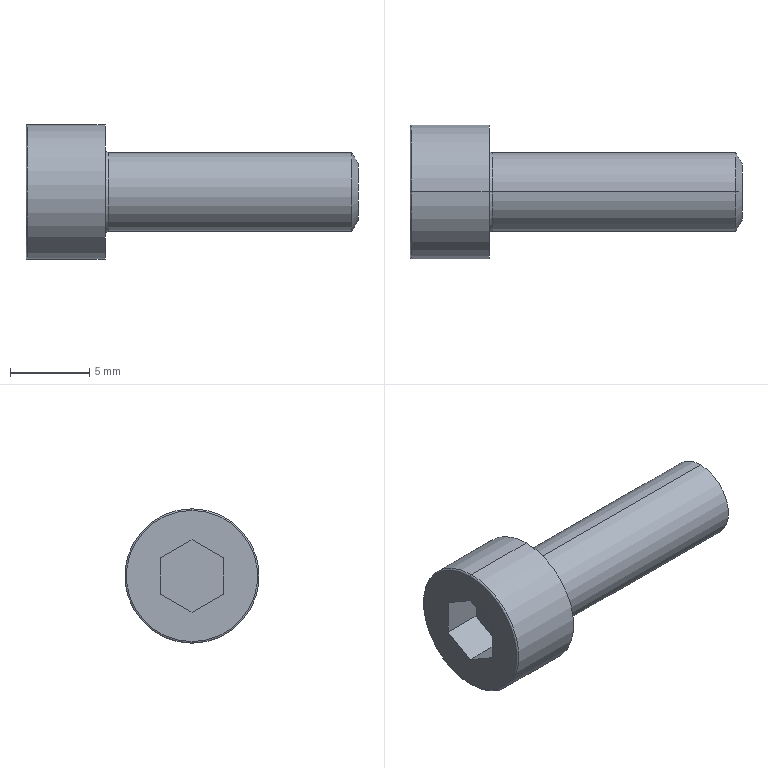Part | SolidWorks | features BlendCut 1, Cut 1, Fillet 1, LPattern 1, RevCut 1, Revolution 1 | 1 solid | 20 faces | box 21 x 8.5 x 8.5 mm | volume 561.928 mm3 | plane 10 | torus 4 | cylinder 4 | cone 2 | commonest cylinder face diameters 5 x2 8.5 x2
STEP:
#1=CARTESIAN_POINT('',(0.,0.,4.15));
#2=VERTEX_POINT('',#1);
#3=CARTESIAN_POINT('',(0.,0.,-4.15));
#4=VERTEX_POINT('',#3);
#5=CARTESIAN_POINT('',(0.,0.,0.));
#6=DIRECTION('',(-1.,0.,0.));
#7=DIRECTION('',(0.,0.,-1.));
#8=AXIS2_PLACEMENT_3D('',#5,#6,#7);
#9=CIRCLE('',#8,4.15);
#10=EDGE_CURVE('',#2,#4,#9,.T.);
#11=ORIENTED_EDGE('',*,*,#10,.F.);
#12=CARTESIAN_POINT('',(0.1,0.,4.25));
#13=VERTEX_POINT('',#12);
#14=CARTESIAN_POINT('',(0.1,0.,4.15));
#15=DIRECTION('',(0.,1.,0.));
#16=DIRECTION('',(0.,0.,1.));
#17=AXIS2_PLACEMENT_3D('',#14,#15,#16);
#18=CIRCLE('',#17,0.1);
#19=EDGE_CURVE('',#2,#13,#18,.T.);
#20=ORIENTED_EDGE('',*,*,#19,.T.);
#21=CARTESIAN_POINT('',(0.1,0.,-4.25));
#22=VERTEX_POINT('',#21);
#23=CARTESIAN_POINT('',(0.1,0.,0.));
#24=DIRECTION('',(1.,0.,0.));
#25=DIRECTION('',(0.,0.,-1.));
#26=AXIS2_PLACEMENT_3D('',#23,#24,#25);
#27=CIRCLE('',#26,4.25);
#28=EDGE_CURVE('',#22,#13,#27,.T.);
#29=ORIENTED_EDGE('',*,*,#28,.F.);
#30=CARTESIAN_POINT('',(0.1,0.,-4.15));
#31=DIRECTION('',(0.,-1.,0.));
#32=DIRECTION('',(0.,0.,-1.));
#33=AXIS2_PLACEMENT_3D('',#30,#31,#32);
#34=CIRCLE('',#33,0.1);
#35=EDGE_CURVE('',#4,#22,#34,.T.);
#36=ORIENTED_EDGE('',*,*,#35,.F.);
#37=EDGE_LOOP('',(#11,#20,#29,#36));
#38=FACE_OUTER_BOUND('',#37,.T.);
#39=CARTESIAN_POINT('',(0.1,0.,0.));
#40=DIRECTION('',(1.,0.,0.));
#41=DIRECTION('',(0.,0.,-1.));
#42=AXIS2_PLACEMENT_3D('',#39,#40,#41);
#43=TOROIDAL_SURFACE('',#42,4.15,0.1);
#44=ADVANCED_FACE('',(#38),#43,.T.);
#45=CARTESIAN_POINT('',(21.,0.,1.807));
#46=VERTEX_POINT('',#45);
#47=CARTESIAN_POINT('',(21.,0.,-1.807));
#48=VERTEX_POINT('',#47);
#49=CARTESIAN_POINT('',(21.,0.,0.));
#50=DIRECTION('',(-1.,0.,0.));
#51=DIRECTION('',(0.,0.,1.));
#52=AXIS2_PLACEMENT_3D('',#49,#50,#51);
#53=CIRCLE('',#52,1.807);
#54=EDGE_CURVE('',#46,#48,#53,.T.);
#55=ORIENTED_EDGE('',*,*,#54,.T.);
#56=CARTESIAN_POINT('',(20.6,0.,-2.5));
#57=VERTEX_POINT('',#56);
#58=CARTESIAN_POINT('',(20.6,0.,-2.5));
#59=DIRECTION('',(-0.5,0.,-0.866));
#60=VECTOR('',#59,1000.);
#61=LINE('',#58,#60);
#62=EDGE_CURVE('',#48,#57,#61,.T.);
#63=ORIENTED_EDGE('',*,*,#62,.T.);
#64=CARTESIAN_POINT('',(20.6,0.,2.5));
#65=VERTEX_POINT('',#64);
#66=CARTESIAN_POINT('',(20.6,0.,0.));
#67=DIRECTION('',(-1.,0.,0.));
#68=DIRECTION('',(0.,0.,1.));
#69=AXIS2_PLACEMENT_3D('',#66,#67,#68);
#70=CIRCLE('',#69,2.5);
#71=EDGE_CURVE('',#65,#57,#70,.T.);
#72=ORIENTED_EDGE('',*,*,#71,.F.);
#73=CARTESIAN_POINT('',(20.6,0.,2.5));
#74=DIRECTION('',(-0.5,0.,0.866));
#75=VECTOR('',#74,1000.);
#76=LINE('',#73,#75);
#77=EDGE_CURVE('',#46,#65,#76,.T.);
#78=ORIENTED_EDGE('',*,*,#77,.F.);
#79=EDGE_LOOP('',(#55,#63,#72,#78));
#80=FACE_OUTER_BOUND('',#79,.T.);
#81=CARTESIAN_POINT('',(20.6,0.,0.));
#82=DIRECTION('',(-1.,0.,0.));
#83=DIRECTION('',(0.,0.,1.));
#84=AXIS2_PLACEMENT_3D('',#81,#82,#83);
#85=CONICAL_SURFACE('',#84,2.5,1.047);
#86=ADVANCED_FACE('',(#80),#85,.T.);
#87=CARTESIAN_POINT('',(5.,0.,-2.7));
#88=VERTEX_POINT('',#87);
#89=CARTESIAN_POINT('',(5.,0.,2.7));
#90=VERTEX_POINT('',#89);
#91=CARTESIAN_POINT('',(5.,0.,0.));
#92=DIRECTION('',(-1.,0.,0.));
#93=DIRECTION('',(0.,0.,1.));
#94=AXIS2_PLACEMENT_3D('',#91,#92,#93);
#95=CIRCLE('',#94,2.7);
#96=EDGE_CURVE('',#88,#90,#95,.T.);
#97=ORIENTED_EDGE('',*,*,#96,.F.);
#98=CARTESIAN_POINT('',(5.2,0.,-2.5));
#99=VERTEX_POINT('',#98);
#100=CARTESIAN_POINT('',(5.2,0.,-2.7));
#101=DIRECTION('',(0.,1.,0.));
#102=DIRECTION('',(0.,0.,1.));
#103=AXIS2_PLACEMENT_3D('',#100,#101,#102);
#104=CIRCLE('',#103,0.2);
#105=EDGE_CURVE('',#88,#99,#104,.T.);
#106=ORIENTED_EDGE('',*,*,#105,.T.);
#107=CARTESIAN_POINT('',(5.2,0.,2.5));
#108=VERTEX_POINT('',#107);
#109=CARTESIAN_POINT('',(5.2,0.,0.));
#110=DIRECTION('',(-1.,0.,0.));
#111=DIRECTION('',(0.,0.,1.));
#112=AXIS2_PLACEMENT_3D('',#109,#110,#111);
#113=CIRCLE('',#112,2.5);
#114=EDGE_CURVE('',#99,#108,#113,.T.);
#115=ORIENTED_EDGE('',*,*,#114,.T.);
#116=CARTESIAN_POINT('',(5.2,0.,2.7));
#117=DIRECTION('',(0.,-1.,0.));
#118=DIRECTION('',(0.,0.,-1.));
#119=AXIS2_PLACEMENT_3D('',#116,#117,#118);
#120=CIRCLE('',#119,0.2);
#121=EDGE_CURVE('',#90,#108,#120,.T.);
#122=ORIENTED_EDGE('',*,*,#121,.F.);
#123=EDGE_LOOP('',(#97,#106,#115,#122));
#124=FACE_OUTER_BOUND('',#123,.T.);
#125=CARTESIAN_POINT('',(5.2,0.,0.));
#126=DIRECTION('',(-1.,0.,0.));
#127=DIRECTION('',(0.,0.,1.));
#128=AXIS2_PLACEMENT_3D('',#125,#126,#127);
#129=TOROIDAL_SURFACE('',#128,2.7,0.2);
#130=ADVANCED_FACE('',(#124),#129,.F.);
#131=CARTESIAN_POINT('',(5.,0.,4.25));
#132=VERTEX_POINT('',#131);
#133=CARTESIAN_POINT('',(5.,0.,-4.25));
#134=VERTEX_POINT('',#133);
#135=CARTESIAN_POINT('',(5.,0.,0.));
#136=DIRECTION('',(-1.,0.,0.));
#137=DIRECTION('',(0.,0.,1.));
#138=AXIS2_PLACEMENT_3D('',#135,#136,#137);
#139=CIRCLE('',#138,4.25);
#140=EDGE_CURVE('',#132,#134,#139,.T.);
#141=ORIENTED_EDGE('',*,*,#140,.T.);
#142=CARTESIAN_POINT('',(0.,0.,-4.25));
#143=DIRECTION('',(-1.,0.,0.));
#144=VECTOR('',#143,1000.);
#145=LINE('',#142,#144);
#146=EDGE_CURVE('',#134,#22,#145,.T.);
#147=ORIENTED_EDGE('',*,*,#146,.T.);
#148=ORIENTED_EDGE('',*,*,#28,.T.);
#149=CARTESIAN_POINT('',(0.,0.,4.25));
#150=DIRECTION('',(-1.,0.,0.));
#151=VECTOR('',#150,1000.);
#152=LINE('',#149,#151);
#153=EDGE_CURVE('',#132,#13,#152,.T.);
#154=ORIENTED_EDGE('',*,*,#153,.F.);
#155=EDGE_LOOP('',(#141,#147,#148,#154));
#156=FACE_OUTER_BOUND('',#155,.T.);
#157=CARTESIAN_POINT('',(0.,0.,0.));
#158=DIRECTION('',(-1.,0.,0.));
#159=DIRECTION('',(0.,0.,1.));
#160=AXIS2_PLACEMENT_3D('',#157,#158,#159);
#161=CYLINDRICAL_SURFACE('',#160,4.25);
#162=ADVANCED_FACE('',(#156),#161,.T.);
#163=ORIENTED_EDGE('',*,*,#71,.T.);
#164=CARTESIAN_POINT('',(0.,0.,-2.5));
#165=DIRECTION('',(-1.,0.,0.));
#166=VECTOR('',#165,1000.);
#167=LINE('',#164,#166);
#168=EDGE_CURVE('',#57,#99,#167,.T.);
#169=ORIENTED_EDGE('',*,*,#168,.T.);
#170=CARTESIAN_POINT('',(5.2,0.,0.));
#171=DIRECTION('',(-1.,0.,0.));
#172=DIRECTION('',(0.,0.,1.));
#173=AXIS2_PLACEMENT_3D('',#170,#171,#172);
#174=CIRCLE('',#173,2.5);
#175=EDGE_CURVE('',#108,#99,#174,.T.);
#176=ORIENTED_EDGE('',*,*,#175,.F.);
#177=CARTESIAN_POINT('',(0.,0.,2.5));
#178=DIRECTION('',(-1.,0.,0.));
#179=VECTOR('',#178,1000.);
#180=LINE('',#177,#179);
#181=EDGE_CURVE('',#65,#108,#180,.T.);
#182=ORIENTED_EDGE('',*,*,#181,.F.);
#183=EDGE_LOOP('',(#163,#169,#176,#182));
#184=FACE_OUTER_BOUND('',#183,.T.);
#185=CARTESIAN_POINT('',(0.,0.,0.));
#186=DIRECTION('',(-1.,0.,0.));
#187=DIRECTION('',(0.,0.,1.));
#188=AXIS2_PLACEMENT_3D('',#185,#186,#187);
#189=CYLINDRICAL_SURFACE('',#188,2.5);
#190=ADVANCED_FACE('',(#184),#189,.T.);
#191=ORIENTED_EDGE('',*,*,#168,.F.);
#192=CARTESIAN_POINT('',(20.6,0.,0.));
#193=DIRECTION('',(-1.,0.,0.));
#194=DIRECTION('',(0.,0.,1.));
#195=AXIS2_PLACEMENT_3D('',#192,#193,#194);
#196=CIRCLE('',#195,2.5);
#197=EDGE_CURVE('',#57,#65,#196,.T.);
#198=ORIENTED_EDGE('',*,*,#197,.T.);
#199=ORIENTED_EDGE('',*,*,#181,.T.);
#200=ORIENTED_EDGE('',*,*,#114,.F.);
#201=EDGE_LOOP('',(#191,#198,#199,#200));
#202=FACE_OUTER_BOUND('',#201,.T.);
#203=CARTESIAN_POINT('',(0.,0.,0.));
#204=DIRECTION('',(-1.,0.,0.));
#205=DIRECTION('',(0.,0.,1.));
#206=AXIS2_PLACEMENT_3D('',#203,#204,#205);
#207=CYLINDRICAL_SURFACE('',#206,2.5);
#208=ADVANCED_FACE('',(#202),#207,.T.);
#209=CARTESIAN_POINT('',(0.,0.,0.));
#210=DIRECTION('',(-1.,0.,0.));
#211=DIRECTION('',(0.,0.,-1.));
#212=AXIS2_PLACEMENT_3D('',#209,#210,#211);
#213=CIRCLE('',#212,4.15);
#214=EDGE_CURVE('',#4,#2,#213,.T.);
#215=ORIENTED_EDGE('',*,*,#214,.T.);
#216=ORIENTED_EDGE('',*,*,#10,.T.);
#217=EDGE_LOOP('',(#215,#216));
#218=FACE_OUTER_BOUND('',#217,.T.);
#219=CARTESIAN_POINT('',(0.,0.,2.29));
#220=VERTEX_POINT('',#219);
#221=CARTESIAN_POINT('',(0.,1.983,1.145));
#222=VERTEX_POINT('',#221);
#223=CARTESIAN_POINT('',(0.,0.,2.29));
#224=DIRECTION('',(0.,0.866,-0.5));
#225=VECTOR('',#224,1000.);
#226=LINE('',#223,#225);
#227=EDGE_CURVE('',#220,#222,#226,.T.);
#228=ORIENTED_EDGE('',*,*,#227,.F.);
#229=CARTESIAN_POINT('',(0.,-1.983,1.145));
#230=VERTEX_POINT('',#229);
#231=CARTESIAN_POINT('',(0.,-1.983,1.145));
#232=DIRECTION('',(0.,0.866,0.5));
#233=VECTOR('',#232,1000.);
#234=LINE('',#231,#233);
#235=EDGE_CURVE('',#230,#220,#234,.T.);
#236=ORIENTED_EDGE('',*,*,#235,.F.);
#237=CARTESIAN_POINT('',(0.,-1.983,-1.145));
#238=VERTEX_POINT('',#237);
#239=CARTESIAN_POINT('',(0.,-1.983,-1.145));
#240=DIRECTION('',(0.,0.,1.));
#241=VECTOR('',#240,1000.);
#242=LINE('',#239,#241);
#243=EDGE_CURVE('',#238,#230,#242,.T.);
#244=ORIENTED_EDGE('',*,*,#243,.F.);
#245=CARTESIAN_POINT('',(0.,0.,-2.29));
#246=VERTEX_POINT('',#245);
#247=CARTESIAN_POINT('',(0.,0.,-2.29));
#248=DIRECTION('',(0.,-0.866,0.5));
#249=VECTOR('',#248,1000.);
#250=LINE('',#247,#249);
#251=EDGE_CURVE('',#246,#238,#250,.T.);
#252=ORIENTED_EDGE('',*,*,#251,.F.);
#253=CARTESIAN_POINT('',(0.,1.983,-1.145));
#254=VERTEX_POINT('',#253);
#255=CARTESIAN_POINT('',(0.,1.983,-1.145));
#256=DIRECTION('',(0.,-0.866,-0.5));
#257=VECTOR('',#256,1000.);
#258=LINE('',#255,#257);
#259=EDGE_CURVE('',#254,#246,#258,.T.);
#260=ORIENTED_EDGE('',*,*,#259,.F.);
#261=CARTESIAN_POINT('',(0.,1.983,1.145));
#262=DIRECTION('',(0.,0.,-1.));
#263=VECTOR('',#262,1000.);
#264=LINE('',#261,#263);
#265=EDGE_CURVE('',#222,#254,#264,.T.);
#266=ORIENTED_EDGE('',*,*,#265,.F.);
#267=EDGE_LOOP('',(#228,#236,#244,#252,#260,#266));
#268=FACE_BOUND('',#267,.T.);
#269=CARTESIAN_POINT('',(0.,0.,0.));
#270=DIRECTION('',(1.,0.,0.));
#271=DIRECTION('',(0.,0.,-1.));
#272=AXIS2_PLACEMENT_3D('',#269,#270,#271);
#273=PLANE('',#272);
#274=ADVANCED_FACE('',(#218,#268),#273,.F.);
#275=ORIENTED_EDGE('',*,*,#146,.F.);
#276=CARTESIAN_POINT('',(5.,0.,0.));
#277=DIRECTION('',(-1.,0.,0.));
#278=DIRECTION('',(0.,0.,1.));
#279=AXIS2_PLACEMENT_3D('',#276,#277,#278);
#280=CIRCLE('',#279,4.25);
#281=EDGE_CURVE('',#134,#132,#280,.T.);
#282=ORIENTED_EDGE('',*,*,#281,.T.);
#283=ORIENTED_EDGE('',*,*,#153,.T.);
#284=CARTESIAN_POINT('',(0.1,0.,0.));
#285=DIRECTION('',(1.,0.,0.));
#286=DIRECTION('',(0.,0.,-1.));
#287=AXIS2_PLACEMENT_3D('',#284,#285,#286);
#288=CIRCLE('',#287,4.25);
#289=EDGE_CURVE('',#13,#22,#288,.T.);
#290=ORIENTED_EDGE('',*,*,#289,.T.);
#291=EDGE_LOOP('',(#275,#282,#283,#290));
#292=FACE_OUTER_BOUND('',#291,.T.);
#293=CARTESIAN_POINT('',(0.,0.,0.));
#294=DIRECTION('',(-1.,0.,0.));
#295=DIRECTION('',(0.,0.,1.));
#296=AXIS2_PLACEMENT_3D('',#293,#294,#295);
#297=CYLINDRICAL_SURFACE('',#296,4.25);
#298=ADVANCED_FACE('',(#292),#297,.T.);
#299=ORIENTED_EDGE('',*,*,#140,.F.);
#300=ORIENTED_EDGE('',*,*,#281,.F.);
#301=EDGE_LOOP('',(#299,#300));
#302=FACE_OUTER_BOUND('',#301,.T.);
#303=CARTESIAN_POINT('',(5.,0.,0.));
#304=DIRECTION('',(-1.,0.,0.));
#305=DIRECTION('',(0.,0.,1.));
#306=AXIS2_PLACEMENT_3D('',#303,#304,#305);
#307=CIRCLE('',#306,2.7);
#308=EDGE_CURVE('',#90,#88,#307,.T.);
#309=ORIENTED_EDGE('',*,*,#308,.T.);
#310=ORIENTED_EDGE('',*,*,#96,.T.);
#311=EDGE_LOOP('',(#309,#310));
#312=FACE_BOUND('',#311,.T.);
#313=CARTESIAN_POINT('',(5.,4.25,0.));
#314=DIRECTION('',(-1.,0.,0.));
#315=DIRECTION('',(0.,0.,1.));
#316=AXIS2_PLACEMENT_3D('',#313,#314,#315);
#317=PLANE('',#316);
#318=ADVANCED_FACE('',(#302,#312),#317,.F.);
#319=ORIENTED_EDGE('',*,*,#105,.F.);
#320=ORIENTED_EDGE('',*,*,#308,.F.);
#321=ORIENTED_EDGE('',*,*,#121,.T.);
#322=ORIENTED_EDGE('',*,*,#175,.T.);
#323=EDGE_LOOP('',(#319,#320,#321,#322));
#324=FACE_OUTER_BOUND('',#323,.T.);
#325=CARTESIAN_POINT('',(5.2,0.,0.));
#326=DIRECTION('',(-1.,0.,0.));
#327=DIRECTION('',(0.,0.,1.));
#328=AXIS2_PLACEMENT_3D('',#325,#326,#327);
#329=TOROIDAL_SURFACE('',#328,2.7,0.2);
#330=ADVANCED_FACE('',(#324),#329,.F.);
#331=ORIENTED_EDGE('',*,*,#235,.T.);
#332=CARTESIAN_POINT('',(2.5,0.,2.29));
#333=VERTEX_POINT('',#332);
#334=CARTESIAN_POINT('',(2.5,0.,2.29));
#335=DIRECTION('',(-1.,0.,0.));
#336=VECTOR('',#335,1000.);
#337=LINE('',#334,#336);
#338=EDGE_CURVE('',#333,#220,#337,.T.);
#339=ORIENTED_EDGE('',*,*,#338,.F.);
#340=CARTESIAN_POINT('',(2.5,-1.983,1.145));
#341=VERTEX_POINT('',#340);
#342=CARTESIAN_POINT('',(2.5,-1.983,1.145));
#343=DIRECTION('',(0.,0.866,0.5));
#344=VECTOR('',#343,1000.);
#345=LINE('',#342,#344);
#346=EDGE_CURVE('',#341,#333,#345,.T.);
#347=ORIENTED_EDGE('',*,*,#346,.F.);
#348=CARTESIAN_POINT('',(2.5,-1.983,1.145));
#349=DIRECTION('',(-1.,0.,0.));
#350=VECTOR('',#349,1000.);
#351=LINE('',#348,#350);
#352=EDGE_CURVE('',#341,#230,#351,.T.);
#353=ORIENTED_EDGE('',*,*,#352,.T.);
#354=EDGE_LOOP('',(#331,#339,#347,#353));
#355=FACE_OUTER_BOUND('',#354,.T.);
#356=CARTESIAN_POINT('',(2.5,-1.983,1.145));
#357=DIRECTION('',(0.,-0.5,0.866));
#358=DIRECTION('',(0.,-0.866,-0.5));
#359=AXIS2_PLACEMENT_3D('',#356,#357,#358);
#360=PLANE('',#359);
#361=ADVANCED_FACE('',(#355),#360,.F.);
#362=ORIENTED_EDGE('',*,*,#243,.T.);
#363=ORIENTED_EDGE('',*,*,#352,.F.);
#364=CARTESIAN_POINT('',(2.5,-1.983,-1.145));
#365=VERTEX_POINT('',#364);
#366=CARTESIAN_POINT('',(2.5,-1.983,-1.145));
#367=DIRECTION('',(0.,0.,1.));
#368=VECTOR('',#367,1000.);
#369=LINE('',#366,#368);
#370=EDGE_CURVE('',#365,#341,#369,.T.);
#371=ORIENTED_EDGE('',*,*,#370,.F.);
#372=CARTESIAN_POINT('',(2.5,-1.983,-1.145));
#373=DIRECTION('',(-1.,0.,0.));
#374=VECTOR('',#373,1000.);
#375=LINE('',#372,#374);
#376=EDGE_CURVE('',#365,#238,#375,.T.);
#377=ORIENTED_EDGE('',*,*,#376,.T.);
#378=EDGE_LOOP('',(#362,#363,#371,#377));
#379=FACE_OUTER_BOUND('',#378,.T.);
#380=CARTESIAN_POINT('',(2.5,-1.983,-1.145));
#381=DIRECTION('',(0.,-1.,0.));
#382=DIRECTION('',(0.,0.,-1.));
#383=AXIS2_PLACEMENT_3D('',#380,#381,#382);
#384=PLANE('',#383);
#385=ADVANCED_FACE('',(#379),#384,.F.);
#386=ORIENTED_EDGE('',*,*,#251,.T.);
#387=ORIENTED_EDGE('',*,*,#376,.F.);
#388=CARTESIAN_POINT('',(2.5,0.,-2.29));
#389=VERTEX_POINT('',#388);
#390=CARTESIAN_POINT('',(2.5,0.,-2.29));
#391=DIRECTION('',(0.,-0.866,0.5));
#392=VECTOR('',#391,1000.);
#393=LINE('',#390,#392);
#394=EDGE_CURVE('',#389,#365,#393,.T.);
#395=ORIENTED_EDGE('',*,*,#394,.F.);
#396=CARTESIAN_POINT('',(2.5,0.,-2.29));
#397=DIRECTION('',(-1.,0.,0.));
#398=VECTOR('',#397,1000.);
#399=LINE('',#396,#398);
#400=EDGE_CURVE('',#389,#246,#399,.T.);
#401=ORIENTED_EDGE('',*,*,#400,.T.);
#402=EDGE_LOOP('',(#386,#387,#395,#401));
#403=FACE_OUTER_BOUND('',#402,.T.);
#404=CARTESIAN_POINT('',(2.5,0.,-2.29));
#405=DIRECTION('',(0.,-0.5,-0.866));
#406=DIRECTION('',(0.,0.866,-0.5));
#407=AXIS2_PLACEMENT_3D('',#404,#405,#406);
#408=PLANE('',#407);
#409=ADVANCED_FACE('',(#403),#408,.F.);
#410=ORIENTED_EDGE('',*,*,#259,.T.);
#411=ORIENTED_EDGE('',*,*,#400,.F.);
#412=CARTESIAN_POINT('',(2.5,1.983,-1.145));
#413=VERTEX_POINT('',#412);
#414=CARTESIAN_POINT('',(2.5,1.983,-1.145));
#415=DIRECTION('',(0.,-0.866,-0.5));
#416=VECTOR('',#415,1000.);
#417=LINE('',#414,#416);
#418=EDGE_CURVE('',#413,#389,#417,.T.);
#419=ORIENTED_EDGE('',*,*,#418,.F.);
#420=CARTESIAN_POINT('',(2.5,1.983,-1.145));
#421=DIRECTION('',(-1.,0.,0.));
#422=VECTOR('',#421,1000.);
#423=LINE('',#420,#422);
#424=EDGE_CURVE('',#413,#254,#423,.T.);
#425=ORIENTED_EDGE('',*,*,#424,.T.);
#426=EDGE_LOOP('',(#410,#411,#419,#425));
#427=FACE_OUTER_BOUND('',#426,.T.);
#428=CARTESIAN_POINT('',(2.5,1.983,-1.145));
#429=DIRECTION('',(0.,0.5,-0.866));
#430=DIRECTION('',(0.,0.866,0.5));
#431=AXIS2_PLACEMENT_3D('',#428,#429,#430);
#432=PLANE('',#431);
#433=ADVANCED_FACE('',(#427),#432,.F.);
#434=ORIENTED_EDGE('',*,*,#265,.T.);
#435=ORIENTED_EDGE('',*,*,#424,.F.);
#436=CARTESIAN_POINT('',(2.5,1.983,1.145));
#437=VERTEX_POINT('',#436);
#438=CARTESIAN_POINT('',(2.5,1.983,1.145));
#439=DIRECTION('',(0.,0.,-1.));
#440=VECTOR('',#439,1000.);
#441=LINE('',#438,#440);
#442=EDGE_CURVE('',#437,#413,#441,.T.);
#443=ORIENTED_EDGE('',*,*,#442,.F.);
#444=CARTESIAN_POINT('',(2.5,1.983,1.145));
#445=DIRECTION('',(-1.,0.,0.));
#446=VECTOR('',#445,1000.);
#447=LINE('',#444,#446);
#448=EDGE_CURVE('',#437,#222,#447,.T.);
#449=ORIENTED_EDGE('',*,*,#448,.T.);
#450=EDGE_LOOP('',(#434,#435,#443,#449));
#451=FACE_OUTER_BOUND('',#450,.T.);
#452=CARTESIAN_POINT('',(2.5,1.983,1.145));
#453=DIRECTION('',(0.,1.,0.));
#454=DIRECTION('',(0.,0.,1.));
#455=AXIS2_PLACEMENT_3D('',#452,#453,#454);
#456=PLANE('',#455);
#457=ADVANCED_FACE('',(#451),#456,.F.);
#458=ORIENTED_EDGE('',*,*,#227,.T.);
#459=ORIENTED_EDGE('',*,*,#448,.F.);
#460=CARTESIAN_POINT('',(2.5,0.,2.29));
#461=DIRECTION('',(0.,0.866,-0.5));
#462=VECTOR('',#461,1000.);
#463=LINE('',#460,#462);
#464=EDGE_CURVE('',#333,#437,#463,.T.);
#465=ORIENTED_EDGE('',*,*,#464,.F.);
#466=ORIENTED_EDGE('',*,*,#338,.T.);
#467=EDGE_LOOP('',(#458,#459,#465,#466));
#468=FACE_OUTER_BOUND('',#467,.T.);
#469=CARTESIAN_POINT('',(2.5,0.,2.29));
#470=DIRECTION('',(0.,0.5,0.866));
#471=DIRECTION('',(0.,-0.866,0.5));
#472=AXIS2_PLACEMENT_3D('',#469,#470,#471);
#473=PLANE('',#472);
#474=ADVANCED_FACE('',(#468),#473,.F.);
#475=ORIENTED_EDGE('',*,*,#346,.T.);
#476=ORIENTED_EDGE('',*,*,#464,.T.);
#477=ORIENTED_EDGE('',*,*,#442,.T.);
#478=ORIENTED_EDGE('',*,*,#418,.T.);
#479=ORIENTED_EDGE('',*,*,#394,.T.);
#480=ORIENTED_EDGE('',*,*,#370,.T.);
#481=EDGE_LOOP('',(#475,#476,#477,#478,#479,#480));
#482=FACE_OUTER_BOUND('',#481,.T.);
#483=CARTESIAN_POINT('',(2.5,-1.983,1.145));
#484=DIRECTION('',(1.,0.,0.));
#485=DIRECTION('',(0.,0.,-1.));
#486=AXIS2_PLACEMENT_3D('',#483,#484,#485);
#487=PLANE('',#486);
#488=ADVANCED_FACE('',(#482),#487,.F.);
#489=ORIENTED_EDGE('',*,*,#62,.F.);
#490=CARTESIAN_POINT('',(21.,0.,0.));
#491=DIRECTION('',(-1.,0.,0.));
#492=DIRECTION('',(0.,0.,1.));
#493=AXIS2_PLACEMENT_3D('',#490,#491,#492);
#494=CIRCLE('',#493,1.807);
#495=EDGE_CURVE('',#48,#46,#494,.T.);
#496=ORIENTED_EDGE('',*,*,#495,.T.);
#497=ORIENTED_EDGE('',*,*,#77,.T.);
#498=ORIENTED_EDGE('',*,*,#197,.F.);
#499=EDGE_LOOP('',(#489,#496,#497,#498));
#500=FACE_OUTER_BOUND('',#499,.T.);
#501=CARTESIAN_POINT('',(20.6,0.,0.));
#502=DIRECTION('',(-1.,0.,0.));
#503=DIRECTION('',(0.,0.,1.));
#504=AXIS2_PLACEMENT_3D('',#501,#502,#503);
#505=CONICAL_SURFACE('',#504,2.5,1.047);
#506=ADVANCED_FACE('',(#500),#505,.T.);
#507=ORIENTED_EDGE('',*,*,#54,.F.);
#508=ORIENTED_EDGE('',*,*,#495,.F.);
#509=EDGE_LOOP('',(#507,#508));
#510=FACE_OUTER_BOUND('',#509,.T.);
#511=CARTESIAN_POINT('',(21.,2.5,0.));
#512=DIRECTION('',(-1.,0.,0.));
#513=DIRECTION('',(0.,0.,1.));
#514=AXIS2_PLACEMENT_3D('',#511,#512,#513);
#515=PLANE('',#514);
#516=ADVANCED_FACE('',(#510),#515,.F.);
#517=ORIENTED_EDGE('',*,*,#19,.F.);
#518=ORIENTED_EDGE('',*,*,#214,.F.);
#519=ORIENTED_EDGE('',*,*,#35,.T.);
#520=ORIENTED_EDGE('',*,*,#289,.F.);
#521=EDGE_LOOP('',(#517,#518,#519,#520));
#522=FACE_OUTER_BOUND('',#521,.T.);
#523=CARTESIAN_POINT('',(0.1,0.,0.));
#524=DIRECTION('',(1.,0.,0.));
#525=DIRECTION('',(0.,0.,-1.));
#526=AXIS2_PLACEMENT_3D('',#523,#524,#525);
#527=TOROIDAL_SURFACE('',#526,4.15,0.1);
#528=ADVANCED_FACE('',(#522),#527,.T.);
#529=CLOSED_SHELL('',(#44,#86,#130,#162,#190,#208,#274,#298,#318,#330,#361,#385,#409,#433,#457,#474,#488,#506,#516,#528));
#530=MANIFOLD_SOLID_BREP('',#529);
#531=CARTESIAN_POINT('',(0.,0.,0.));
#532=DIRECTION('',(0.,0.,1.));
#533=DIRECTION('',(1.,0.,0.));
#534=AXIS2_PLACEMENT_3D('',#531,#532,#533);
#535=(LENGTH_UNIT()NAMED_UNIT(*)SI_UNIT(.MILLI.,.METRE.));
#536=UNCERTAINTY_MEASURE_WITH_UNIT(LENGTH_MEASURE(0.00001),#535,'','');
#537=(NAMED_UNIT(*)PLANE_ANGLE_UNIT()SI_UNIT($,.RADIAN.));
#538=(NAMED_UNIT(*)SI_UNIT($,.STERADIAN.)SOLID_ANGLE_UNIT());
#539=(GEOMETRIC_REPRESENTATION_CONTEXT(3)GLOBAL_UNCERTAINTY_ASSIGNED_CONTEXT((#536))GLOBAL_UNIT_ASSIGNED_CONTEXT((#535,#537,#538))REPRESENTATION_CONTEXT('',''));
#540=ADVANCED_BREP_SHAPE_REPRESENTATION('',(#530,#534),#539);